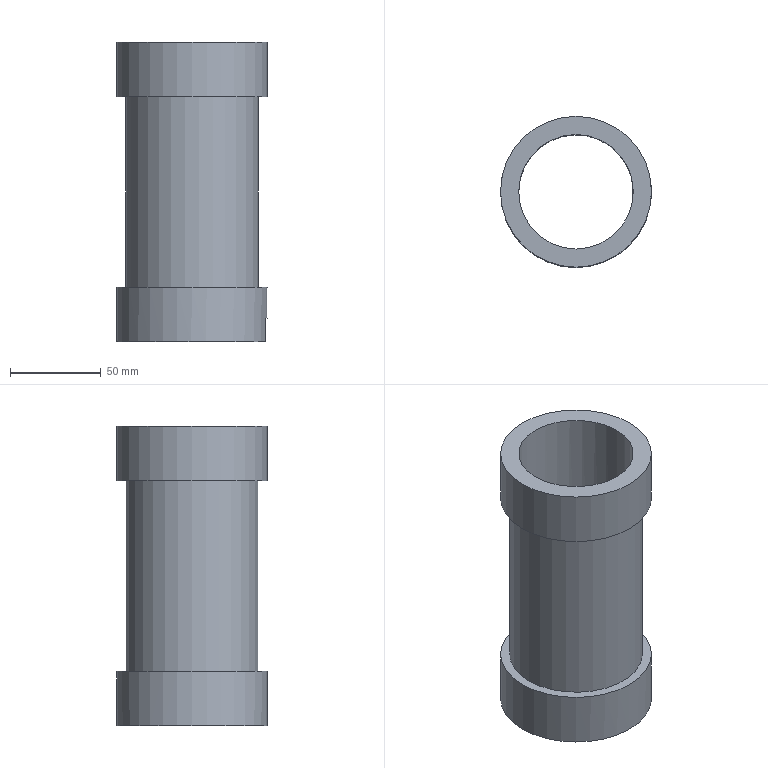Part | NX | features ACO1640-04 2 | 1 solid | 12 faces | box 83 x 83 x 165 mm | volume 247016 mm3 | plane 7 | cylinder 5 | commonest cylinder face diameters 83 x2 6.917 x1 63 x1 73 x1
STEP:
#1=CARTESIAN_POINT('',(-866.965,681.389,-73.342));
#2=VERTEX_POINT('',#1);
#3=CARTESIAN_POINT('',(-868.923,681.519,-71.321));
#4=CARTESIAN_POINT('',(-866.636,681.369,-73.162));
#5=CARTESIAN_POINT('',(-866.324,681.337,-76.081));
#6=CARTESIAN_POINT('',(-868.16,681.486,-78.361));
#7=CARTESIAN_POINT('',(-871.077,681.519,-78.679));
#8=CARTESIAN_POINT('',(-873.364,681.369,-76.838));
#9=CARTESIAN_POINT('',(-873.676,681.337,-73.919));
#10=CARTESIAN_POINT('',(-871.84,681.486,-71.639));
#11=CARTESIAN_POINT('',(-868.923,681.519,-71.321));
#12=CARTESIAN_POINT('',(-866.636,681.369,-73.162));
#13=CARTESIAN_POINT('',(-866.324,681.337,-76.081));
#14=B_SPLINE_CURVE_WITH_KNOTS('',3,(#3,#4,#5,#6,#7,#8,#9,#10,#11,#12,#13),.UNSPECIFIED.,.T.,.F.,(1,1,1,1,1,1,1,1,1,1,1,1,1,1,1),(-0.008112,-0.005408,-0.002704,0.,0.002704,0.005408,0.008112,0.01082,0.01352,0.01622,0.01893,0.02163,0.02433,0.02704,0.02974),.UNSPECIFIED.);
#15=EDGE_CURVE('',#2,#2,#14,.T.);
#16=ORIENTED_EDGE('',*,*,#15,.T.);
#17=EDGE_LOOP('',(#16));
#18=FACE_BOUND('',#17,.T.);
#19=CARTESIAN_POINT('',(-873.035,671.353,-76.658));
#20=VERTEX_POINT('',#19);
#21=CARTESIAN_POINT('',(-873.677,671.285,-73.915));
#22=CARTESIAN_POINT('',(-873.363,671.328,-76.839));
#23=CARTESIAN_POINT('',(-871.08,671.525,-78.677));
#24=CARTESIAN_POINT('',(-868.165,671.482,-78.364));
#25=CARTESIAN_POINT('',(-866.323,671.285,-76.085));
#26=CARTESIAN_POINT('',(-866.636,671.328,-73.161));
#27=CARTESIAN_POINT('',(-868.92,671.525,-71.323));
#28=CARTESIAN_POINT('',(-871.835,671.482,-71.636));
#29=CARTESIAN_POINT('',(-873.677,671.285,-73.915));
#30=CARTESIAN_POINT('',(-873.363,671.328,-76.839));
#31=CARTESIAN_POINT('',(-871.08,671.525,-78.677));
#32=B_SPLINE_CURVE_WITH_KNOTS('',3,(#21,#22,#23,#24,#25,#26,#27,#28,#29,#30,#31),.UNSPECIFIED.,.T.,.F.,(1,1,1,1,1,1,1,1,1,1,1,1,1,1,1),(-0.008114,-0.005409,-0.002705,0.,0.002705,0.005409,0.008114,0.01082,0.01352,0.01623,0.01893,0.02164,0.02434,0.02705,0.02975),.UNSPECIFIED.);
#33=EDGE_CURVE('',#20,#20,#32,.T.);
#34=ORIENTED_EDGE('',*,*,#33,.T.);
#35=EDGE_LOOP('',(#34));
#36=FACE_BOUND('',#35,.T.);
#37=CARTESIAN_POINT('',(-870.,681.4,-75.));
#38=DIRECTION('',(0.,-1.,0.));
#39=DIRECTION('',(1.,0.,0.));
#40=AXIS2_PLACEMENT_3D('',#37,#38,#39);
#41=CYLINDRICAL_SURFACE('',#40,3.458);
#42=ADVANCED_FACE('',(#18,#36),#41,.F.);
#43=CARTESIAN_POINT('',(-911.5,640.,-65.));
#44=VERTEX_POINT('',#43);
#45=CARTESIAN_POINT('',(-870.,640.,-65.));
#46=DIRECTION('',(0.,0.,-1.));
#47=DIRECTION('',(-1.,0.,0.));
#48=AXIS2_PLACEMENT_3D('',#45,#46,#47);
#49=CIRCLE('',#48,41.5);
#50=EDGE_CURVE('',#44,#44,#49,.T.);
#51=ORIENTED_EDGE('',*,*,#50,.T.);
#52=EDGE_LOOP('',(#51));
#53=FACE_BOUND('',#52,.T.);
#54=CARTESIAN_POINT('',(-829.488,631.,-95.));
#55=VERTEX_POINT('',#54);
#56=CARTESIAN_POINT('',(-829.488,649.,-95.));
#57=VERTEX_POINT('',#56);
#58=CARTESIAN_POINT('',(-870.,640.,-95.));
#59=DIRECTION('',(0.,0.,-1.));
#60=DIRECTION('',(-1.,0.,0.));
#61=AXIS2_PLACEMENT_3D('',#58,#59,#60);
#62=CIRCLE('',#61,41.5);
#63=EDGE_CURVE('',#55,#57,#62,.T.);
#64=ORIENTED_EDGE('',*,*,#63,.F.);
#65=CARTESIAN_POINT('',(-829.488,631.,-82.));
#66=VERTEX_POINT('',#65);
#67=CARTESIAN_POINT('',(-829.488,631.,-88.5));
#68=DIRECTION('',(0.,0.,-1.));
#69=VECTOR('',#68,1000.);
#70=LINE('',#67,#69);
#71=EDGE_CURVE('',#66,#55,#70,.T.);
#72=ORIENTED_EDGE('',*,*,#71,.F.);
#73=CARTESIAN_POINT('',(-829.488,649.,-82.));
#74=VERTEX_POINT('',#73);
#75=CARTESIAN_POINT('',(-870.,640.,-82.));
#76=DIRECTION('',(0.,0.,1.));
#77=DIRECTION('',(1.,0.,0.));
#78=AXIS2_PLACEMENT_3D('',#75,#76,#77);
#79=CIRCLE('',#78,41.5);
#80=EDGE_CURVE('',#66,#74,#79,.T.);
#81=ORIENTED_EDGE('',*,*,#80,.T.);
#82=CARTESIAN_POINT('',(-829.488,649.,-88.5));
#83=DIRECTION('',(0.,0.,1.));
#84=VECTOR('',#83,1000.);
#85=LINE('',#82,#84);
#86=EDGE_CURVE('',#57,#74,#85,.T.);
#87=ORIENTED_EDGE('',*,*,#86,.F.);
#88=EDGE_LOOP('',(#64,#72,#81,#87));
#89=FACE_BOUND('',#88,.T.);
#90=ORIENTED_EDGE('',*,*,#15,.F.);
#91=EDGE_LOOP('',(#90));
#92=FACE_BOUND('',#91,.T.);
#93=CARTESIAN_POINT('',(-870.,640.,-12.5));
#94=DIRECTION('',(0.,0.,-1.));
#95=DIRECTION('',(-1.,0.,0.));
#96=AXIS2_PLACEMENT_3D('',#93,#94,#95);
#97=CYLINDRICAL_SURFACE('',#96,41.5);
#98=ADVANCED_FACE('',(#53,#89,#92),#97,.T.);
#99=CARTESIAN_POINT('',(-839.813,631.,-95.));
#100=VERTEX_POINT('',#99);
#101=CARTESIAN_POINT('',(-839.813,649.,-95.));
#102=VERTEX_POINT('',#101);
#103=CARTESIAN_POINT('',(-870.,640.,-95.));
#104=DIRECTION('',(0.,0.,-1.));
#105=DIRECTION('',(-1.,0.,0.));
#106=AXIS2_PLACEMENT_3D('',#103,#104,#105);
#107=CIRCLE('',#106,31.5);
#108=EDGE_CURVE('',#100,#102,#107,.T.);
#109=ORIENTED_EDGE('',*,*,#108,.T.);
#110=CARTESIAN_POINT('',(-839.813,649.,-82.));
#111=VERTEX_POINT('',#110);
#112=CARTESIAN_POINT('',(-839.813,649.,-88.5));
#113=DIRECTION('',(0.,0.,1.));
#114=VECTOR('',#113,1000.);
#115=LINE('',#112,#114);
#116=EDGE_CURVE('',#102,#111,#115,.T.);
#117=ORIENTED_EDGE('',*,*,#116,.T.);
#118=CARTESIAN_POINT('',(-839.813,631.,-82.));
#119=VERTEX_POINT('',#118);
#120=CARTESIAN_POINT('',(-870.,640.,-82.));
#121=DIRECTION('',(0.,0.,1.));
#122=DIRECTION('',(1.,0.,0.));
#123=AXIS2_PLACEMENT_3D('',#120,#121,#122);
#124=CIRCLE('',#123,31.5);
#125=EDGE_CURVE('',#119,#111,#124,.T.);
#126=ORIENTED_EDGE('',*,*,#125,.F.);
#127=CARTESIAN_POINT('',(-839.813,631.,-88.5));
#128=DIRECTION('',(0.,0.,1.));
#129=VECTOR('',#128,1000.);
#130=LINE('',#127,#129);
#131=EDGE_CURVE('',#100,#119,#130,.T.);
#132=ORIENTED_EDGE('',*,*,#131,.F.);
#133=EDGE_LOOP('',(#109,#117,#126,#132));
#134=FACE_BOUND('',#133,.T.);
#135=CARTESIAN_POINT('',(-901.5,640.,70.));
#136=VERTEX_POINT('',#135);
#137=CARTESIAN_POINT('',(-870.,640.,70.));
#138=DIRECTION('',(0.,0.,-1.));
#139=DIRECTION('',(-1.,0.,0.));
#140=AXIS2_PLACEMENT_3D('',#137,#138,#139);
#141=CIRCLE('',#140,31.5);
#142=EDGE_CURVE('',#136,#136,#141,.T.);
#143=ORIENTED_EDGE('',*,*,#142,.F.);
#144=EDGE_LOOP('',(#143));
#145=FACE_BOUND('',#144,.T.);
#146=ORIENTED_EDGE('',*,*,#33,.F.);
#147=EDGE_LOOP('',(#146));
#148=FACE_BOUND('',#147,.T.);
#149=CARTESIAN_POINT('',(-870.,640.,-12.5));
#150=DIRECTION('',(0.,0.,-1.));
#151=DIRECTION('',(-1.,0.,0.));
#152=AXIS2_PLACEMENT_3D('',#149,#150,#151);
#153=CYLINDRICAL_SURFACE('',#152,31.5);
#154=ADVANCED_FACE('',(#134,#145,#148),#153,.F.);
#155=ORIENTED_EDGE('',*,*,#50,.F.);
#156=EDGE_LOOP('',(#155));
#157=FACE_BOUND('',#156,.T.);
#158=CARTESIAN_POINT('',(-906.5,640.,-65.));
#159=VERTEX_POINT('',#158);
#160=CARTESIAN_POINT('',(-870.,640.,-65.));
#161=DIRECTION('',(0.,0.,-1.));
#162=DIRECTION('',(-1.,0.,0.));
#163=AXIS2_PLACEMENT_3D('',#160,#161,#162);
#164=CIRCLE('',#163,36.5);
#165=EDGE_CURVE('',#159,#159,#164,.T.);
#166=ORIENTED_EDGE('',*,*,#165,.T.);
#167=EDGE_LOOP('',(#166));
#168=FACE_BOUND('',#167,.T.);
#169=CARTESIAN_POINT('',(-870.,676.5,-65.));
#170=DIRECTION('',(0.,0.,-1.));
#171=DIRECTION('',(-1.,0.,0.));
#172=AXIS2_PLACEMENT_3D('',#169,#170,#171);
#173=PLANE('',#172);
#174=ADVANCED_FACE('',(#157,#168),#173,.F.);
#175=CARTESIAN_POINT('',(-906.5,640.,40.));
#176=VERTEX_POINT('',#175);
#177=CARTESIAN_POINT('',(-870.,640.,40.));
#178=DIRECTION('',(0.,0.,-1.));
#179=DIRECTION('',(-1.,0.,0.));
#180=AXIS2_PLACEMENT_3D('',#177,#178,#179);
#181=CIRCLE('',#180,36.5);
#182=EDGE_CURVE('',#176,#176,#181,.T.);
#183=ORIENTED_EDGE('',*,*,#182,.T.);
#184=EDGE_LOOP('',(#183));
#185=FACE_BOUND('',#184,.T.);
#186=ORIENTED_EDGE('',*,*,#165,.F.);
#187=EDGE_LOOP('',(#186));
#188=FACE_BOUND('',#187,.T.);
#189=CARTESIAN_POINT('',(-870.,640.,-12.5));
#190=DIRECTION('',(0.,0.,-1.));
#191=DIRECTION('',(-1.,0.,0.));
#192=AXIS2_PLACEMENT_3D('',#189,#190,#191);
#193=CYLINDRICAL_SURFACE('',#192,36.5);
#194=ADVANCED_FACE('',(#185,#188),#193,.T.);
#195=CARTESIAN_POINT('',(-911.5,640.,40.));
#196=VERTEX_POINT('',#195);
#197=CARTESIAN_POINT('',(-870.,640.,40.));
#198=DIRECTION('',(0.,0.,-1.));
#199=DIRECTION('',(-1.,0.,0.));
#200=AXIS2_PLACEMENT_3D('',#197,#198,#199);
#201=CIRCLE('',#200,41.5);
#202=EDGE_CURVE('',#196,#196,#201,.T.);
#203=ORIENTED_EDGE('',*,*,#202,.T.);
#204=EDGE_LOOP('',(#203));
#205=FACE_BOUND('',#204,.T.);
#206=ORIENTED_EDGE('',*,*,#182,.F.);
#207=EDGE_LOOP('',(#206));
#208=FACE_BOUND('',#207,.T.);
#209=CARTESIAN_POINT('',(-870.,681.5,40.));
#210=DIRECTION('',(0.,0.,-1.));
#211=DIRECTION('',(-1.,0.,0.));
#212=AXIS2_PLACEMENT_3D('',#209,#210,#211);
#213=PLANE('',#212);
#214=ADVANCED_FACE('',(#205,#208),#213,.T.);
#215=CARTESIAN_POINT('',(-911.5,640.,70.));
#216=VERTEX_POINT('',#215);
#217=CARTESIAN_POINT('',(-870.,640.,70.));
#218=DIRECTION('',(0.,0.,-1.));
#219=DIRECTION('',(-1.,0.,0.));
#220=AXIS2_PLACEMENT_3D('',#217,#218,#219);
#221=CIRCLE('',#220,41.5);
#222=EDGE_CURVE('',#216,#216,#221,.T.);
#223=ORIENTED_EDGE('',*,*,#222,.T.);
#224=EDGE_LOOP('',(#223));
#225=FACE_BOUND('',#224,.T.);
#226=ORIENTED_EDGE('',*,*,#202,.F.);
#227=EDGE_LOOP('',(#226));
#228=FACE_BOUND('',#227,.T.);
#229=CARTESIAN_POINT('',(-870.,640.,-12.5));
#230=DIRECTION('',(0.,0.,-1.));
#231=DIRECTION('',(-1.,0.,0.));
#232=AXIS2_PLACEMENT_3D('',#229,#230,#231);
#233=CYLINDRICAL_SURFACE('',#232,41.5);
#234=ADVANCED_FACE('',(#225,#228),#233,.T.);
#235=CARTESIAN_POINT('',(-834.65,649.,-82.));
#236=DIRECTION('',(1.,0.,0.));
#237=VECTOR('',#236,1000.);
#238=LINE('',#235,#237);
#239=EDGE_CURVE('',#111,#74,#238,.T.);
#240=ORIENTED_EDGE('',*,*,#239,.T.);
#241=ORIENTED_EDGE('',*,*,#80,.F.);
#242=CARTESIAN_POINT('',(-834.65,631.,-82.));
#243=DIRECTION('',(1.,0.,0.));
#244=VECTOR('',#243,1000.);
#245=LINE('',#242,#244);
#246=EDGE_CURVE('',#119,#66,#245,.T.);
#247=ORIENTED_EDGE('',*,*,#246,.F.);
#248=ORIENTED_EDGE('',*,*,#125,.T.);
#249=EDGE_LOOP('',(#240,#241,#247,#248));
#250=FACE_BOUND('',#249,.T.);
#251=CARTESIAN_POINT('',(-870.,649.,-82.));
#252=DIRECTION('',(0.,0.,1.));
#253=DIRECTION('',(1.,0.,0.));
#254=AXIS2_PLACEMENT_3D('',#251,#252,#253);
#255=PLANE('',#254);
#256=ADVANCED_FACE('',(#250),#255,.F.);
#257=ORIENTED_EDGE('',*,*,#246,.T.);
#258=ORIENTED_EDGE('',*,*,#71,.T.);
#259=CARTESIAN_POINT('',(-834.65,631.,-95.));
#260=DIRECTION('',(1.,0.,0.));
#261=VECTOR('',#260,1000.);
#262=LINE('',#259,#261);
#263=EDGE_CURVE('',#100,#55,#262,.T.);
#264=ORIENTED_EDGE('',*,*,#263,.F.);
#265=ORIENTED_EDGE('',*,*,#131,.T.);
#266=EDGE_LOOP('',(#257,#258,#264,#265));
#267=FACE_BOUND('',#266,.T.);
#268=CARTESIAN_POINT('',(-870.,631.,-82.));
#269=DIRECTION('',(0.,-1.,0.));
#270=DIRECTION('',(0.,0.,-1.));
#271=AXIS2_PLACEMENT_3D('',#268,#269,#270);
#272=PLANE('',#271);
#273=ADVANCED_FACE('',(#267),#272,.F.);
#274=CARTESIAN_POINT('',(-834.65,649.,-95.));
#275=DIRECTION('',(1.,0.,0.));
#276=VECTOR('',#275,1000.);
#277=LINE('',#274,#276);
#278=EDGE_CURVE('',#102,#57,#277,.T.);
#279=ORIENTED_EDGE('',*,*,#278,.T.);
#280=ORIENTED_EDGE('',*,*,#86,.T.);
#281=ORIENTED_EDGE('',*,*,#239,.F.);
#282=ORIENTED_EDGE('',*,*,#116,.F.);
#283=EDGE_LOOP('',(#279,#280,#281,#282));
#284=FACE_BOUND('',#283,.T.);
#285=CARTESIAN_POINT('',(-870.,649.,-95.));
#286=DIRECTION('',(0.,1.,0.));
#287=DIRECTION('',(0.,0.,1.));
#288=AXIS2_PLACEMENT_3D('',#285,#286,#287);
#289=PLANE('',#288);
#290=ADVANCED_FACE('',(#284),#289,.F.);
#291=ORIENTED_EDGE('',*,*,#222,.F.);
#292=EDGE_LOOP('',(#291));
#293=FACE_BOUND('',#292,.T.);
#294=ORIENTED_EDGE('',*,*,#142,.T.);
#295=EDGE_LOOP('',(#294));
#296=FACE_BOUND('',#295,.T.);
#297=CARTESIAN_POINT('',(-870.,671.5,70.));
#298=DIRECTION('',(0.,0.,-1.));
#299=DIRECTION('',(-1.,0.,0.));
#300=AXIS2_PLACEMENT_3D('',#297,#298,#299);
#301=PLANE('',#300);
#302=ADVANCED_FACE('',(#293,#296),#301,.F.);
#303=ORIENTED_EDGE('',*,*,#263,.T.);
#304=ORIENTED_EDGE('',*,*,#63,.T.);
#305=ORIENTED_EDGE('',*,*,#278,.F.);
#306=ORIENTED_EDGE('',*,*,#108,.F.);
#307=EDGE_LOOP('',(#303,#304,#305,#306));
#308=FACE_BOUND('',#307,.T.);
#309=CARTESIAN_POINT('',(-870.,671.5,-95.));
#310=DIRECTION('',(0.,0.,-1.));
#311=DIRECTION('',(-1.,0.,0.));
#312=AXIS2_PLACEMENT_3D('',#309,#310,#311);
#313=PLANE('',#312);
#314=ADVANCED_FACE('',(#308),#313,.T.);
#315=CLOSED_SHELL('',(#42,#98,#154,#174,#194,#214,#234,#256,#273,#290,#302,#314));
#316=MANIFOLD_SOLID_BREP('',#315);
#317=(LENGTH_UNIT()NAMED_UNIT(*)SI_UNIT(.MILLI.,.METRE.));
#318=UNCERTAINTY_MEASURE_WITH_UNIT(LENGTH_MEASURE(0.0508),#317,'','');
#319=(NAMED_UNIT(*)PLANE_ANGLE_UNIT()SI_UNIT($,.RADIAN.));
#320=(NAMED_UNIT(*)SI_UNIT($,.STERADIAN.)SOLID_ANGLE_UNIT());
#321=(GEOMETRIC_REPRESENTATION_CONTEXT(3)GLOBAL_UNCERTAINTY_ASSIGNED_CONTEXT((#318))GLOBAL_UNIT_ASSIGNED_CONTEXT((#317,#319,#320))REPRESENTATION_CONTEXT('',''));
#322=ADVANCED_BREP_SHAPE_REPRESENTATION('',(#316),#321);